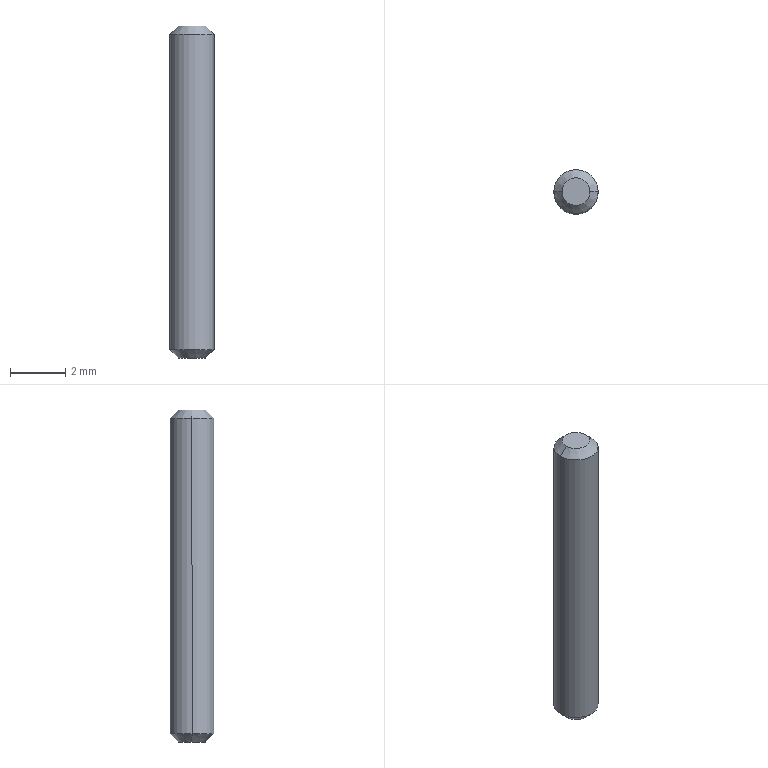Part | STEP file | 1 solid | 8 faces | box 1.6 x 1.6 x 12 mm | volume 23.732 mm3 | cone 4 | cylinder 2 | plane 2 | commonest cylinder face diameters 1.6 x2
STEP:
#1=CARTESIAN_POINT('',(-0.8,0.,11.7));
#2=VERTEX_POINT('',#1);
#3=CARTESIAN_POINT('',(0.8,0.,11.7));
#4=VERTEX_POINT('',#3);
#5=CARTESIAN_POINT('',(0.,0.,11.7));
#6=DIRECTION('',(0.,0.,-1.));
#7=DIRECTION('',(-1.,0.,0.));
#8=AXIS2_PLACEMENT_3D('',#5,#6,#7);
#9=CIRCLE('',#8,0.8);
#10=EDGE_CURVE('',#2,#4,#9,.T.);
#11=ORIENTED_EDGE('',*,*,#10,.T.);
#12=CARTESIAN_POINT('',(0.8,0.,0.3));
#13=VERTEX_POINT('',#12);
#14=CARTESIAN_POINT('',(0.8,0.,12.));
#15=DIRECTION('',(0.,0.,-1.));
#16=VECTOR('',#15,1000.);
#17=LINE('',#14,#16);
#18=EDGE_CURVE('',#4,#13,#17,.T.);
#19=ORIENTED_EDGE('',*,*,#18,.T.);
#20=CARTESIAN_POINT('',(-0.8,0.,0.3));
#21=VERTEX_POINT('',#20);
#22=CARTESIAN_POINT('',(0.,0.,0.3));
#23=DIRECTION('',(0.,0.,1.));
#24=DIRECTION('',(-1.,0.,0.));
#25=AXIS2_PLACEMENT_3D('',#22,#23,#24);
#26=CIRCLE('',#25,0.8);
#27=EDGE_CURVE('',#13,#21,#26,.T.);
#28=ORIENTED_EDGE('',*,*,#27,.T.);
#29=CARTESIAN_POINT('',(-0.8,0.,12.));
#30=DIRECTION('',(0.,0.,-1.));
#31=VECTOR('',#30,1000.);
#32=LINE('',#29,#31);
#33=EDGE_CURVE('',#2,#21,#32,.T.);
#34=ORIENTED_EDGE('',*,*,#33,.F.);
#35=EDGE_LOOP('',(#11,#19,#28,#34));
#36=FACE_OUTER_BOUND('',#35,.T.);
#37=CARTESIAN_POINT('',(0.,0.,12.));
#38=DIRECTION('',(0.,0.,-1.));
#39=DIRECTION('',(-1.,0.,0.));
#40=AXIS2_PLACEMENT_3D('',#37,#38,#39);
#41=CYLINDRICAL_SURFACE('',#40,0.8);
#42=ADVANCED_FACE('',(#36),#41,.T.);
#43=CARTESIAN_POINT('',(0.5,0.,0.));
#44=VERTEX_POINT('',#43);
#45=CARTESIAN_POINT('',(-0.5,0.,0.));
#46=VERTEX_POINT('',#45);
#47=CARTESIAN_POINT('',(0.,0.,0.));
#48=DIRECTION('',(0.,0.,1.));
#49=DIRECTION('',(1.,0.,0.));
#50=AXIS2_PLACEMENT_3D('',#47,#48,#49);
#51=CIRCLE('',#50,0.5);
#52=EDGE_CURVE('',#44,#46,#51,.T.);
#53=ORIENTED_EDGE('',*,*,#52,.T.);
#54=CARTESIAN_POINT('',(-0.8,0.,0.3));
#55=DIRECTION('',(-0.7071,0.,0.7071));
#56=VECTOR('',#55,1000.);
#57=LINE('',#54,#56);
#58=EDGE_CURVE('',#46,#21,#57,.T.);
#59=ORIENTED_EDGE('',*,*,#58,.T.);
#60=ORIENTED_EDGE('',*,*,#27,.F.);
#61=CARTESIAN_POINT('',(0.8,0.,0.3));
#62=DIRECTION('',(0.7071,0.,0.7071));
#63=VECTOR('',#62,1000.);
#64=LINE('',#61,#63);
#65=EDGE_CURVE('',#44,#13,#64,.T.);
#66=ORIENTED_EDGE('',*,*,#65,.F.);
#67=EDGE_LOOP('',(#53,#59,#60,#66));
#68=FACE_OUTER_BOUND('',#67,.T.);
#69=CARTESIAN_POINT('',(0.,0.,0.3));
#70=DIRECTION('',(0.,0.,1.));
#71=DIRECTION('',(1.,0.,0.));
#72=AXIS2_PLACEMENT_3D('',#69,#70,#71);
#73=CONICAL_SURFACE('',#72,0.8,0.7854);
#74=ADVANCED_FACE('',(#68),#73,.T.);
#75=CARTESIAN_POINT('',(-0.5,0.,12.));
#76=VERTEX_POINT('',#75);
#77=CARTESIAN_POINT('',(0.5,0.,12.));
#78=VERTEX_POINT('',#77);
#79=CARTESIAN_POINT('',(0.,0.,12.));
#80=DIRECTION('',(0.,0.,-1.));
#81=DIRECTION('',(-1.,0.,0.));
#82=AXIS2_PLACEMENT_3D('',#79,#80,#81);
#83=CIRCLE('',#82,0.5);
#84=EDGE_CURVE('',#76,#78,#83,.T.);
#85=ORIENTED_EDGE('',*,*,#84,.T.);
#86=CARTESIAN_POINT('',(0.8,0.,11.7));
#87=DIRECTION('',(0.7071,0.,-0.7071));
#88=VECTOR('',#87,1000.);
#89=LINE('',#86,#88);
#90=EDGE_CURVE('',#78,#4,#89,.T.);
#91=ORIENTED_EDGE('',*,*,#90,.T.);
#92=ORIENTED_EDGE('',*,*,#10,.F.);
#93=CARTESIAN_POINT('',(-0.8,0.,11.7));
#94=DIRECTION('',(-0.7071,0.,-0.7071));
#95=VECTOR('',#94,1000.);
#96=LINE('',#93,#95);
#97=EDGE_CURVE('',#76,#2,#96,.T.);
#98=ORIENTED_EDGE('',*,*,#97,.F.);
#99=EDGE_LOOP('',(#85,#91,#92,#98));
#100=FACE_OUTER_BOUND('',#99,.T.);
#101=CARTESIAN_POINT('',(0.,0.,11.7));
#102=DIRECTION('',(0.,0.,-1.));
#103=DIRECTION('',(-1.,0.,0.));
#104=AXIS2_PLACEMENT_3D('',#101,#102,#103);
#105=CONICAL_SURFACE('',#104,0.8,0.7854);
#106=ADVANCED_FACE('',(#100),#105,.T.);
#107=ORIENTED_EDGE('',*,*,#18,.F.);
#108=CARTESIAN_POINT('',(0.,0.,11.7));
#109=DIRECTION('',(0.,0.,-1.));
#110=DIRECTION('',(-1.,0.,0.));
#111=AXIS2_PLACEMENT_3D('',#108,#109,#110);
#112=CIRCLE('',#111,0.8);
#113=EDGE_CURVE('',#4,#2,#112,.T.);
#114=ORIENTED_EDGE('',*,*,#113,.T.);
#115=ORIENTED_EDGE('',*,*,#33,.T.);
#116=CARTESIAN_POINT('',(0.,0.,0.3));
#117=DIRECTION('',(0.,0.,1.));
#118=DIRECTION('',(-1.,0.,0.));
#119=AXIS2_PLACEMENT_3D('',#116,#117,#118);
#120=CIRCLE('',#119,0.8);
#121=EDGE_CURVE('',#21,#13,#120,.T.);
#122=ORIENTED_EDGE('',*,*,#121,.T.);
#123=EDGE_LOOP('',(#107,#114,#115,#122));
#124=FACE_OUTER_BOUND('',#123,.T.);
#125=CARTESIAN_POINT('',(0.,0.,12.));
#126=DIRECTION('',(0.,0.,-1.));
#127=DIRECTION('',(-1.,0.,0.));
#128=AXIS2_PLACEMENT_3D('',#125,#126,#127);
#129=CYLINDRICAL_SURFACE('',#128,0.8);
#130=ADVANCED_FACE('',(#124),#129,.T.);
#131=ORIENTED_EDGE('',*,*,#58,.F.);
#132=CARTESIAN_POINT('',(0.,0.,0.));
#133=DIRECTION('',(0.,0.,1.));
#134=DIRECTION('',(1.,0.,0.));
#135=AXIS2_PLACEMENT_3D('',#132,#133,#134);
#136=CIRCLE('',#135,0.5);
#137=EDGE_CURVE('',#46,#44,#136,.T.);
#138=ORIENTED_EDGE('',*,*,#137,.T.);
#139=ORIENTED_EDGE('',*,*,#65,.T.);
#140=ORIENTED_EDGE('',*,*,#121,.F.);
#141=EDGE_LOOP('',(#131,#138,#139,#140));
#142=FACE_OUTER_BOUND('',#141,.T.);
#143=CARTESIAN_POINT('',(0.,0.,0.3));
#144=DIRECTION('',(0.,0.,1.));
#145=DIRECTION('',(1.,0.,0.));
#146=AXIS2_PLACEMENT_3D('',#143,#144,#145);
#147=CONICAL_SURFACE('',#146,0.8,0.7854);
#148=ADVANCED_FACE('',(#142),#147,.T.);
#149=ORIENTED_EDGE('',*,*,#90,.F.);
#150=CARTESIAN_POINT('',(0.,0.,12.));
#151=DIRECTION('',(0.,0.,-1.));
#152=DIRECTION('',(-1.,0.,0.));
#153=AXIS2_PLACEMENT_3D('',#150,#151,#152);
#154=CIRCLE('',#153,0.5);
#155=EDGE_CURVE('',#78,#76,#154,.T.);
#156=ORIENTED_EDGE('',*,*,#155,.T.);
#157=ORIENTED_EDGE('',*,*,#97,.T.);
#158=ORIENTED_EDGE('',*,*,#113,.F.);
#159=EDGE_LOOP('',(#149,#156,#157,#158));
#160=FACE_OUTER_BOUND('',#159,.T.);
#161=CARTESIAN_POINT('',(0.,0.,11.7));
#162=DIRECTION('',(0.,0.,-1.));
#163=DIRECTION('',(-1.,0.,0.));
#164=AXIS2_PLACEMENT_3D('',#161,#162,#163);
#165=CONICAL_SURFACE('',#164,0.8,0.7854);
#166=ADVANCED_FACE('',(#160),#165,.T.);
#167=ORIENTED_EDGE('',*,*,#52,.F.);
#168=ORIENTED_EDGE('',*,*,#137,.F.);
#169=EDGE_LOOP('',(#167,#168));
#170=FACE_OUTER_BOUND('',#169,.T.);
#171=CARTESIAN_POINT('',(0.,0.,0.));
#172=DIRECTION('',(0.,0.,1.));
#173=DIRECTION('',(1.,0.,0.));
#174=AXIS2_PLACEMENT_3D('',#171,#172,#173);
#175=PLANE('',#174);
#176=ADVANCED_FACE('',(#170),#175,.F.);
#177=ORIENTED_EDGE('',*,*,#84,.F.);
#178=ORIENTED_EDGE('',*,*,#155,.F.);
#179=EDGE_LOOP('',(#177,#178));
#180=FACE_OUTER_BOUND('',#179,.T.);
#181=CARTESIAN_POINT('',(0.,0.,12.));
#182=DIRECTION('',(0.,0.,1.));
#183=DIRECTION('',(1.,0.,0.));
#184=AXIS2_PLACEMENT_3D('',#181,#182,#183);
#185=PLANE('',#184);
#186=ADVANCED_FACE('',(#180),#185,.T.);
#187=CLOSED_SHELL('',(#42,#74,#106,#130,#148,#166,#176,#186));
#188=MANIFOLD_SOLID_BREP('',#187);
#189=CARTESIAN_POINT('',(0.,0.,0.));
#190=DIRECTION('',(0.,0.,1.));
#191=DIRECTION('',(1.,0.,0.));
#192=AXIS2_PLACEMENT_3D('',#189,#190,#191);
#193=(LENGTH_UNIT()NAMED_UNIT(*)SI_UNIT(.MILLI.,.METRE.));
#194=UNCERTAINTY_MEASURE_WITH_UNIT(LENGTH_MEASURE(0.00001),#193,'','');
#195=(NAMED_UNIT(*)PLANE_ANGLE_UNIT()SI_UNIT($,.RADIAN.));
#196=(NAMED_UNIT(*)SI_UNIT($,.STERADIAN.)SOLID_ANGLE_UNIT());
#197=(GEOMETRIC_REPRESENTATION_CONTEXT(3)GLOBAL_UNCERTAINTY_ASSIGNED_CONTEXT((#194))GLOBAL_UNIT_ASSIGNED_CONTEXT((#193,#195,#196))REPRESENTATION_CONTEXT('',''));
#198=ADVANCED_BREP_SHAPE_REPRESENTATION('',(#188,#192),#197);